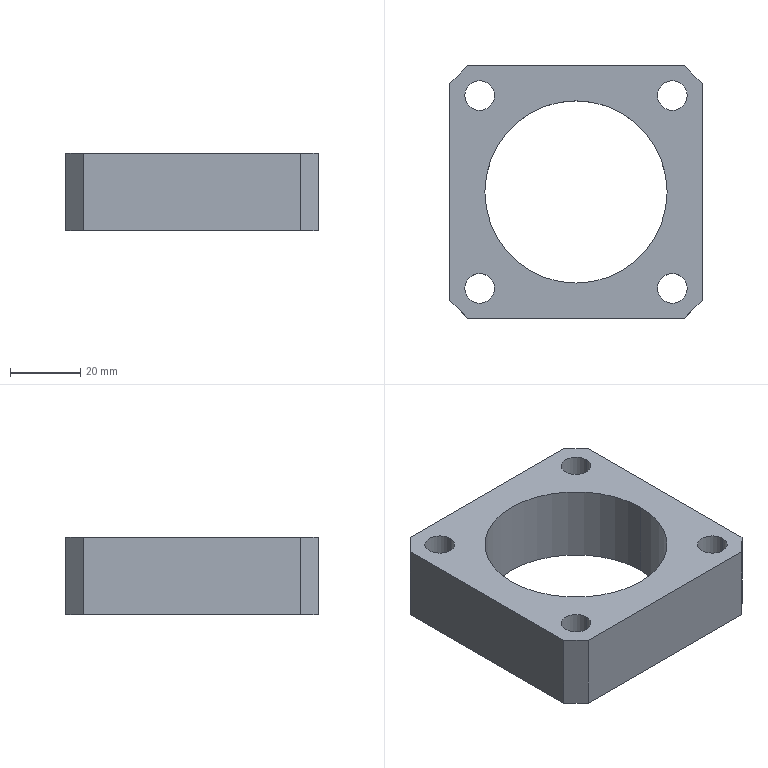Part | 1 solid | 32 faces | box 72 x 72 x 22 mm | volume 58801 mm3 | cylinder 18 | plane 14 | commonest cylinder face diameters 8.5 x8 13 x8 52 x2
STEP:
#1=CARTESIAN_POINT('',(34.,-27.5,-3.));
#2=VERTEX_POINT('',#1);
#3=CARTESIAN_POINT('',(21.,-27.5,-3.));
#4=VERTEX_POINT('',#3);
#5=CARTESIAN_POINT('',(27.5,-27.5,-3.));
#6=DIRECTION('',(0.,0.,-1.));
#7=DIRECTION('',(-1.,0.,0.));
#8=AXIS2_PLACEMENT_3D('',#5,#6,#7);
#9=CIRCLE('',#8,6.5);
#10=EDGE_CURVE('',#2,#4,#9,.T.);
#11=ORIENTED_EDGE('',*,*,#10,.F.);
#12=CARTESIAN_POINT('',(34.,-27.5,-11.));
#13=VERTEX_POINT('',#12);
#14=CARTESIAN_POINT('',(34.,-27.5,-11.));
#15=DIRECTION('',(0.,0.,-1.));
#16=VECTOR('',#15,1000.);
#17=LINE('',#14,#16);
#18=EDGE_CURVE('',#2,#13,#17,.T.);
#19=ORIENTED_EDGE('',*,*,#18,.T.);
#20=CARTESIAN_POINT('',(21.,-27.5,-11.));
#21=VERTEX_POINT('',#20);
#22=CARTESIAN_POINT('',(27.5,-27.5,-11.));
#23=DIRECTION('',(0.,0.,-1.));
#24=DIRECTION('',(-1.,0.,0.));
#25=AXIS2_PLACEMENT_3D('',#22,#23,#24);
#26=CIRCLE('',#25,6.5);
#27=EDGE_CURVE('',#13,#21,#26,.T.);
#28=ORIENTED_EDGE('',*,*,#27,.T.);
#29=CARTESIAN_POINT('',(21.,-27.5,-11.));
#30=DIRECTION('',(0.,0.,-1.));
#31=VECTOR('',#30,1000.);
#32=LINE('',#29,#31);
#33=EDGE_CURVE('',#4,#21,#32,.T.);
#34=ORIENTED_EDGE('',*,*,#33,.F.);
#35=EDGE_LOOP('',(#11,#19,#28,#34));
#36=FACE_OUTER_BOUND('',#35,.T.);
#37=CARTESIAN_POINT('',(27.5,-27.5,-11.));
#38=DIRECTION('',(0.,0.,-1.));
#39=DIRECTION('',(-1.,0.,0.));
#40=AXIS2_PLACEMENT_3D('',#37,#38,#39);
#41=CYLINDRICAL_SURFACE('',#40,6.5);
#42=ADVANCED_FACE('',(#36),#41,.F.);
#43=CARTESIAN_POINT('',(31.75,-27.5,11.));
#44=VERTEX_POINT('',#43);
#45=CARTESIAN_POINT('',(23.25,-27.5,11.));
#46=VERTEX_POINT('',#45);
#47=CARTESIAN_POINT('',(27.5,-27.5,11.));
#48=DIRECTION('',(0.,0.,-1.));
#49=DIRECTION('',(-1.,0.,0.));
#50=AXIS2_PLACEMENT_3D('',#47,#48,#49);
#51=CIRCLE('',#50,4.25);
#52=EDGE_CURVE('',#44,#46,#51,.T.);
#53=ORIENTED_EDGE('',*,*,#52,.F.);
#54=CARTESIAN_POINT('',(31.75,-27.5,-3.));
#55=VERTEX_POINT('',#54);
#56=CARTESIAN_POINT('',(31.75,-27.5,-11.));
#57=DIRECTION('',(0.,0.,-1.));
#58=VECTOR('',#57,1000.);
#59=LINE('',#56,#58);
#60=EDGE_CURVE('',#44,#55,#59,.T.);
#61=ORIENTED_EDGE('',*,*,#60,.T.);
#62=CARTESIAN_POINT('',(23.25,-27.5,-3.));
#63=VERTEX_POINT('',#62);
#64=CARTESIAN_POINT('',(27.5,-27.5,-3.));
#65=DIRECTION('',(0.,0.,-1.));
#66=DIRECTION('',(-1.,0.,0.));
#67=AXIS2_PLACEMENT_3D('',#64,#65,#66);
#68=CIRCLE('',#67,4.25);
#69=EDGE_CURVE('',#55,#63,#68,.T.);
#70=ORIENTED_EDGE('',*,*,#69,.T.);
#71=CARTESIAN_POINT('',(23.25,-27.5,-11.));
#72=DIRECTION('',(0.,0.,-1.));
#73=VECTOR('',#72,1000.);
#74=LINE('',#71,#73);
#75=EDGE_CURVE('',#46,#63,#74,.T.);
#76=ORIENTED_EDGE('',*,*,#75,.F.);
#77=EDGE_LOOP('',(#53,#61,#70,#76));
#78=FACE_OUTER_BOUND('',#77,.T.);
#79=CARTESIAN_POINT('',(27.5,-27.5,-11.));
#80=DIRECTION('',(0.,0.,-1.));
#81=DIRECTION('',(-1.,0.,0.));
#82=AXIS2_PLACEMENT_3D('',#79,#80,#81);
#83=CYLINDRICAL_SURFACE('',#82,4.25);
#84=ADVANCED_FACE('',(#78),#83,.F.);
#85=CARTESIAN_POINT('',(-21.,-27.5,-3.));
#86=VERTEX_POINT('',#85);
#87=CARTESIAN_POINT('',(-34.,-27.5,-3.));
#88=VERTEX_POINT('',#87);
#89=CARTESIAN_POINT('',(-27.5,-27.5,-3.));
#90=DIRECTION('',(0.,0.,-1.));
#91=DIRECTION('',(-1.,0.,0.));
#92=AXIS2_PLACEMENT_3D('',#89,#90,#91);
#93=CIRCLE('',#92,6.5);
#94=EDGE_CURVE('',#86,#88,#93,.T.);
#95=ORIENTED_EDGE('',*,*,#94,.F.);
#96=CARTESIAN_POINT('',(-21.,-27.5,-11.));
#97=VERTEX_POINT('',#96);
#98=CARTESIAN_POINT('',(-21.,-27.5,-11.));
#99=DIRECTION('',(0.,0.,-1.));
#100=VECTOR('',#99,1000.);
#101=LINE('',#98,#100);
#102=EDGE_CURVE('',#86,#97,#101,.T.);
#103=ORIENTED_EDGE('',*,*,#102,.T.);
#104=CARTESIAN_POINT('',(-34.,-27.5,-11.));
#105=VERTEX_POINT('',#104);
#106=CARTESIAN_POINT('',(-27.5,-27.5,-11.));
#107=DIRECTION('',(0.,0.,-1.));
#108=DIRECTION('',(-1.,0.,0.));
#109=AXIS2_PLACEMENT_3D('',#106,#107,#108);
#110=CIRCLE('',#109,6.5);
#111=EDGE_CURVE('',#97,#105,#110,.T.);
#112=ORIENTED_EDGE('',*,*,#111,.T.);
#113=CARTESIAN_POINT('',(-34.,-27.5,-11.));
#114=DIRECTION('',(0.,0.,-1.));
#115=VECTOR('',#114,1000.);
#116=LINE('',#113,#115);
#117=EDGE_CURVE('',#88,#105,#116,.T.);
#118=ORIENTED_EDGE('',*,*,#117,.F.);
#119=EDGE_LOOP('',(#95,#103,#112,#118));
#120=FACE_OUTER_BOUND('',#119,.T.);
#121=CARTESIAN_POINT('',(-27.5,-27.5,-11.));
#122=DIRECTION('',(0.,0.,-1.));
#123=DIRECTION('',(-1.,0.,0.));
#124=AXIS2_PLACEMENT_3D('',#121,#122,#123);
#125=CYLINDRICAL_SURFACE('',#124,6.5);
#126=ADVANCED_FACE('',(#120),#125,.F.);
#127=CARTESIAN_POINT('',(-23.25,-27.5,11.));
#128=VERTEX_POINT('',#127);
#129=CARTESIAN_POINT('',(-31.75,-27.5,11.));
#130=VERTEX_POINT('',#129);
#131=CARTESIAN_POINT('',(-27.5,-27.5,11.));
#132=DIRECTION('',(0.,0.,-1.));
#133=DIRECTION('',(-1.,0.,0.));
#134=AXIS2_PLACEMENT_3D('',#131,#132,#133);
#135=CIRCLE('',#134,4.25);
#136=EDGE_CURVE('',#128,#130,#135,.T.);
#137=ORIENTED_EDGE('',*,*,#136,.F.);
#138=CARTESIAN_POINT('',(-23.25,-27.5,-3.));
#139=VERTEX_POINT('',#138);
#140=CARTESIAN_POINT('',(-23.25,-27.5,-11.));
#141=DIRECTION('',(0.,0.,-1.));
#142=VECTOR('',#141,1000.);
#143=LINE('',#140,#142);
#144=EDGE_CURVE('',#128,#139,#143,.T.);
#145=ORIENTED_EDGE('',*,*,#144,.T.);
#146=CARTESIAN_POINT('',(-31.75,-27.5,-3.));
#147=VERTEX_POINT('',#146);
#148=CARTESIAN_POINT('',(-27.5,-27.5,-3.));
#149=DIRECTION('',(0.,0.,-1.));
#150=DIRECTION('',(-1.,0.,0.));
#151=AXIS2_PLACEMENT_3D('',#148,#149,#150);
#152=CIRCLE('',#151,4.25);
#153=EDGE_CURVE('',#139,#147,#152,.T.);
#154=ORIENTED_EDGE('',*,*,#153,.T.);
#155=CARTESIAN_POINT('',(-31.75,-27.5,-11.));
#156=DIRECTION('',(0.,0.,-1.));
#157=VECTOR('',#156,1000.);
#158=LINE('',#155,#157);
#159=EDGE_CURVE('',#130,#147,#158,.T.);
#160=ORIENTED_EDGE('',*,*,#159,.F.);
#161=EDGE_LOOP('',(#137,#145,#154,#160));
#162=FACE_OUTER_BOUND('',#161,.T.);
#163=CARTESIAN_POINT('',(-27.5,-27.5,-11.));
#164=DIRECTION('',(0.,0.,-1.));
#165=DIRECTION('',(-1.,0.,0.));
#166=AXIS2_PLACEMENT_3D('',#163,#164,#165);
#167=CYLINDRICAL_SURFACE('',#166,4.25);
#168=ADVANCED_FACE('',(#162),#167,.F.);
#169=CARTESIAN_POINT('',(-21.,27.5,-3.));
#170=VERTEX_POINT('',#169);
#171=CARTESIAN_POINT('',(-34.,27.5,-3.));
#172=VERTEX_POINT('',#171);
#173=CARTESIAN_POINT('',(-27.5,27.5,-3.));
#174=DIRECTION('',(0.,0.,-1.));
#175=DIRECTION('',(-1.,0.,0.));
#176=AXIS2_PLACEMENT_3D('',#173,#174,#175);
#177=CIRCLE('',#176,6.5);
#178=EDGE_CURVE('',#170,#172,#177,.T.);
#179=ORIENTED_EDGE('',*,*,#178,.F.);
#180=CARTESIAN_POINT('',(-21.,27.5,-11.));
#181=VERTEX_POINT('',#180);
#182=CARTESIAN_POINT('',(-21.,27.5,-11.));
#183=DIRECTION('',(0.,0.,-1.));
#184=VECTOR('',#183,1000.);
#185=LINE('',#182,#184);
#186=EDGE_CURVE('',#170,#181,#185,.T.);
#187=ORIENTED_EDGE('',*,*,#186,.T.);
#188=CARTESIAN_POINT('',(-34.,27.5,-11.));
#189=VERTEX_POINT('',#188);
#190=CARTESIAN_POINT('',(-27.5,27.5,-11.));
#191=DIRECTION('',(0.,0.,-1.));
#192=DIRECTION('',(-1.,0.,0.));
#193=AXIS2_PLACEMENT_3D('',#190,#191,#192);
#194=CIRCLE('',#193,6.5);
#195=EDGE_CURVE('',#181,#189,#194,.T.);
#196=ORIENTED_EDGE('',*,*,#195,.T.);
#197=CARTESIAN_POINT('',(-34.,27.5,-11.));
#198=DIRECTION('',(0.,0.,-1.));
#199=VECTOR('',#198,1000.);
#200=LINE('',#197,#199);
#201=EDGE_CURVE('',#172,#189,#200,.T.);
#202=ORIENTED_EDGE('',*,*,#201,.F.);
#203=EDGE_LOOP('',(#179,#187,#196,#202));
#204=FACE_OUTER_BOUND('',#203,.T.);
#205=CARTESIAN_POINT('',(-27.5,27.5,-11.));
#206=DIRECTION('',(0.,0.,-1.));
#207=DIRECTION('',(-1.,0.,0.));
#208=AXIS2_PLACEMENT_3D('',#205,#206,#207);
#209=CYLINDRICAL_SURFACE('',#208,6.5);
#210=ADVANCED_FACE('',(#204),#209,.F.);
#211=CARTESIAN_POINT('',(-23.25,27.5,11.));
#212=VERTEX_POINT('',#211);
#213=CARTESIAN_POINT('',(-31.75,27.5,11.));
#214=VERTEX_POINT('',#213);
#215=CARTESIAN_POINT('',(-27.5,27.5,11.));
#216=DIRECTION('',(0.,0.,-1.));
#217=DIRECTION('',(-1.,0.,0.));
#218=AXIS2_PLACEMENT_3D('',#215,#216,#217);
#219=CIRCLE('',#218,4.25);
#220=EDGE_CURVE('',#212,#214,#219,.T.);
#221=ORIENTED_EDGE('',*,*,#220,.F.);
#222=CARTESIAN_POINT('',(-23.25,27.5,-3.));
#223=VERTEX_POINT('',#222);
#224=CARTESIAN_POINT('',(-23.25,27.5,-11.));
#225=DIRECTION('',(0.,0.,-1.));
#226=VECTOR('',#225,1000.);
#227=LINE('',#224,#226);
#228=EDGE_CURVE('',#212,#223,#227,.T.);
#229=ORIENTED_EDGE('',*,*,#228,.T.);
#230=CARTESIAN_POINT('',(-31.75,27.5,-3.));
#231=VERTEX_POINT('',#230);
#232=CARTESIAN_POINT('',(-27.5,27.5,-3.));
#233=DIRECTION('',(0.,0.,-1.));
#234=DIRECTION('',(-1.,0.,0.));
#235=AXIS2_PLACEMENT_3D('',#232,#233,#234);
#236=CIRCLE('',#235,4.25);
#237=EDGE_CURVE('',#223,#231,#236,.T.);
#238=ORIENTED_EDGE('',*,*,#237,.T.);
#239=CARTESIAN_POINT('',(-31.75,27.5,-11.));
#240=DIRECTION('',(0.,0.,-1.));
#241=VECTOR('',#240,1000.);
#242=LINE('',#239,#241);
#243=EDGE_CURVE('',#214,#231,#242,.T.);
#244=ORIENTED_EDGE('',*,*,#243,.F.);
#245=EDGE_LOOP('',(#221,#229,#238,#244));
#246=FACE_OUTER_BOUND('',#245,.T.);
#247=CARTESIAN_POINT('',(-27.5,27.5,-11.));
#248=DIRECTION('',(0.,0.,-1.));
#249=DIRECTION('',(-1.,0.,0.));
#250=AXIS2_PLACEMENT_3D('',#247,#248,#249);
#251=CYLINDRICAL_SURFACE('',#250,4.25);
#252=ADVANCED_FACE('',(#246),#251,.F.);
#253=CARTESIAN_POINT('',(34.,27.5,-3.));
#254=VERTEX_POINT('',#253);
#255=CARTESIAN_POINT('',(21.,27.5,-3.));
#256=VERTEX_POINT('',#255);
#257=CARTESIAN_POINT('',(27.5,27.5,-3.));
#258=DIRECTION('',(0.,0.,-1.));
#259=DIRECTION('',(-1.,0.,0.));
#260=AXIS2_PLACEMENT_3D('',#257,#258,#259);
#261=CIRCLE('',#260,6.5);
#262=EDGE_CURVE('',#254,#256,#261,.T.);
#263=ORIENTED_EDGE('',*,*,#262,.F.);
#264=CARTESIAN_POINT('',(34.,27.5,-11.));
#265=VERTEX_POINT('',#264);
#266=CARTESIAN_POINT('',(34.,27.5,-11.));
#267=DIRECTION('',(0.,0.,-1.));
#268=VECTOR('',#267,1000.);
#269=LINE('',#266,#268);
#270=EDGE_CURVE('',#254,#265,#269,.T.);
#271=ORIENTED_EDGE('',*,*,#270,.T.);
#272=CARTESIAN_POINT('',(21.,27.5,-11.));
#273=VERTEX_POINT('',#272);
#274=CARTESIAN_POINT('',(27.5,27.5,-11.));
#275=DIRECTION('',(0.,0.,-1.));
#276=DIRECTION('',(-1.,0.,0.));
#277=AXIS2_PLACEMENT_3D('',#274,#275,#276);
#278=CIRCLE('',#277,6.5);
#279=EDGE_CURVE('',#265,#273,#278,.T.);
#280=ORIENTED_EDGE('',*,*,#279,.T.);
#281=CARTESIAN_POINT('',(21.,27.5,-11.));
#282=DIRECTION('',(0.,0.,-1.));
#283=VECTOR('',#282,1000.);
#284=LINE('',#281,#283);
#285=EDGE_CURVE('',#256,#273,#284,.T.);
#286=ORIENTED_EDGE('',*,*,#285,.F.);
#287=EDGE_LOOP('',(#263,#271,#280,#286));
#288=FACE_OUTER_BOUND('',#287,.T.);
#289=CARTESIAN_POINT('',(27.5,27.5,-11.));
#290=DIRECTION('',(0.,0.,-1.));
#291=DIRECTION('',(-1.,0.,0.));
#292=AXIS2_PLACEMENT_3D('',#289,#290,#291);
#293=CYLINDRICAL_SURFACE('',#292,6.5);
#294=ADVANCED_FACE('',(#288),#293,.F.);
#295=CARTESIAN_POINT('',(31.75,27.5,11.));
#296=VERTEX_POINT('',#295);
#297=CARTESIAN_POINT('',(23.25,27.5,11.));
#298=VERTEX_POINT('',#297);
#299=CARTESIAN_POINT('',(27.5,27.5,11.));
#300=DIRECTION('',(0.,0.,-1.));
#301=DIRECTION('',(-1.,0.,0.));
#302=AXIS2_PLACEMENT_3D('',#299,#300,#301);
#303=CIRCLE('',#302,4.25);
#304=EDGE_CURVE('',#296,#298,#303,.T.);
#305=ORIENTED_EDGE('',*,*,#304,.F.);
#306=CARTESIAN_POINT('',(31.75,27.5,-3.));
#307=VERTEX_POINT('',#306);
#308=CARTESIAN_POINT('',(31.75,27.5,-11.));
#309=DIRECTION('',(0.,0.,-1.));
#310=VECTOR('',#309,1000.);
#311=LINE('',#308,#310);
#312=EDGE_CURVE('',#296,#307,#311,.T.);
#313=ORIENTED_EDGE('',*,*,#312,.T.);
#314=CARTESIAN_POINT('',(23.25,27.5,-3.));
#315=VERTEX_POINT('',#314);
#316=CARTESIAN_POINT('',(27.5,27.5,-3.));
#317=DIRECTION('',(0.,0.,-1.));
#318=DIRECTION('',(-1.,0.,0.));
#319=AXIS2_PLACEMENT_3D('',#316,#317,#318);
#320=CIRCLE('',#319,4.25);
#321=EDGE_CURVE('',#307,#315,#320,.T.);
#322=ORIENTED_EDGE('',*,*,#321,.T.);
#323=CARTESIAN_POINT('',(23.25,27.5,-11.));
#324=DIRECTION('',(0.,0.,-1.));
#325=VECTOR('',#324,1000.);
#326=LINE('',#323,#325);
#327=EDGE_CURVE('',#298,#315,#326,.T.);
#328=ORIENTED_EDGE('',*,*,#327,.F.);
#329=EDGE_LOOP('',(#305,#313,#322,#328));
#330=FACE_OUTER_BOUND('',#329,.T.);
#331=CARTESIAN_POINT('',(27.5,27.5,-11.));
#332=DIRECTION('',(0.,0.,-1.));
#333=DIRECTION('',(-1.,0.,0.));
#334=AXIS2_PLACEMENT_3D('',#331,#332,#333);
#335=CYLINDRICAL_SURFACE('',#334,4.25);
#336=ADVANCED_FACE('',(#330),#335,.F.);
#337=CARTESIAN_POINT('',(26.,0.,11.));
#338=VERTEX_POINT('',#337);
#339=CARTESIAN_POINT('',(-26.,0.,11.));
#340=VERTEX_POINT('',#339);
#341=CARTESIAN_POINT('',(0.,0.,11.));
#342=DIRECTION('',(0.,0.,-1.));
#343=DIRECTION('',(-1.,0.,0.));
#344=AXIS2_PLACEMENT_3D('',#341,#342,#343);
#345=CIRCLE('',#344,26.);
#346=EDGE_CURVE('',#338,#340,#345,.T.);
#347=ORIENTED_EDGE('',*,*,#346,.F.);
#348=CARTESIAN_POINT('',(26.,0.,-11.));
#349=VERTEX_POINT('',#348);
#350=CARTESIAN_POINT('',(26.,0.,-11.));
#351=DIRECTION('',(0.,0.,-1.));
#352=VECTOR('',#351,1000.);
#353=LINE('',#350,#352);
#354=EDGE_CURVE('',#338,#349,#353,.T.);
#355=ORIENTED_EDGE('',*,*,#354,.T.);
#356=CARTESIAN_POINT('',(-26.,0.,-11.));
#357=VERTEX_POINT('',#356);
#358=CARTESIAN_POINT('',(0.,0.,-11.));
#359=DIRECTION('',(0.,0.,-1.));
#360=DIRECTION('',(-1.,0.,0.));
#361=AXIS2_PLACEMENT_3D('',#358,#359,#360);
#362=CIRCLE('',#361,26.);
#363=EDGE_CURVE('',#349,#357,#362,.T.);
#364=ORIENTED_EDGE('',*,*,#363,.T.);
#365=CARTESIAN_POINT('',(-26.,0.,-11.));
#366=DIRECTION('',(0.,0.,-1.));
#367=VECTOR('',#366,1000.);
#368=LINE('',#365,#367);
#369=EDGE_CURVE('',#340,#357,#368,.T.);
#370=ORIENTED_EDGE('',*,*,#369,.F.);
#371=EDGE_LOOP('',(#347,#355,#364,#370));
#372=FACE_OUTER_BOUND('',#371,.T.);
#373=CARTESIAN_POINT('',(0.,0.,-11.));
#374=DIRECTION('',(0.,0.,-1.));
#375=DIRECTION('',(-1.,0.,0.));
#376=AXIS2_PLACEMENT_3D('',#373,#374,#375);
#377=CYLINDRICAL_SURFACE('',#376,26.);
#378=ADVANCED_FACE('',(#372),#377,.F.);
#379=CARTESIAN_POINT('',(-31.,36.,-11.));
#380=VERTEX_POINT('',#379);
#381=CARTESIAN_POINT('',(31.,36.,-11.));
#382=VERTEX_POINT('',#381);
#383=CARTESIAN_POINT('',(-36.,36.,-11.));
#384=DIRECTION('',(1.,0.,0.));
#385=VECTOR('',#384,1000.);
#386=LINE('',#383,#385);
#387=EDGE_CURVE('',#380,#382,#386,.T.);
#388=ORIENTED_EDGE('',*,*,#387,.F.);
#389=CARTESIAN_POINT('',(-31.,36.,11.));
#390=VERTEX_POINT('',#389);
#391=CARTESIAN_POINT('',(-31.,36.,11.));
#392=DIRECTION('',(0.,0.,1.));
#393=VECTOR('',#392,1000.);
#394=LINE('',#391,#393);
#395=EDGE_CURVE('',#380,#390,#394,.T.);
#396=ORIENTED_EDGE('',*,*,#395,.T.);
#397=CARTESIAN_POINT('',(31.,36.,11.));
#398=VERTEX_POINT('',#397);
#399=CARTESIAN_POINT('',(-36.,36.,11.));
#400=DIRECTION('',(1.,0.,0.));
#401=VECTOR('',#400,1000.);
#402=LINE('',#399,#401);
#403=EDGE_CURVE('',#390,#398,#402,.T.);
#404=ORIENTED_EDGE('',*,*,#403,.T.);
#405=CARTESIAN_POINT('',(31.,36.,11.));
#406=DIRECTION('',(0.,0.,-1.));
#407=VECTOR('',#406,1000.);
#408=LINE('',#405,#407);
#409=EDGE_CURVE('',#398,#382,#408,.T.);
#410=ORIENTED_EDGE('',*,*,#409,.T.);
#411=EDGE_LOOP('',(#388,#396,#404,#410));
#412=FACE_OUTER_BOUND('',#411,.T.);
#413=CARTESIAN_POINT('',(-36.,36.,11.));
#414=DIRECTION('',(0.,1.,0.));
#415=DIRECTION('',(0.,0.,1.));
#416=AXIS2_PLACEMENT_3D('',#413,#414,#415);
#417=PLANE('',#416);
#418=ADVANCED_FACE('',(#412),#417,.T.);
#419=CARTESIAN_POINT('',(-36.,-31.,-11.));
#420=VERTEX_POINT('',#419);
#421=CARTESIAN_POINT('',(-36.,31.,-11.));
#422=VERTEX_POINT('',#421);
#423=CARTESIAN_POINT('',(-36.,-36.,-11.));
#424=DIRECTION('',(0.,1.,0.));
#425=VECTOR('',#424,1000.);
#426=LINE('',#423,#425);
#427=EDGE_CURVE('',#420,#422,#426,.T.);
#428=ORIENTED_EDGE('',*,*,#427,.F.);
#429=CARTESIAN_POINT('',(-36.,-31.,11.));
#430=VERTEX_POINT('',#429);
#431=CARTESIAN_POINT('',(-36.,-31.,11.));
#432=DIRECTION('',(0.,0.,1.));
#433=VECTOR('',#432,1000.);
#434=LINE('',#431,#433);
#435=EDGE_CURVE('',#420,#430,#434,.T.);
#436=ORIENTED_EDGE('',*,*,#435,.T.);
#437=CARTESIAN_POINT('',(-36.,31.,11.));
#438=VERTEX_POINT('',#437);
#439=CARTESIAN_POINT('',(-36.,-36.,11.));
#440=DIRECTION('',(0.,1.,0.));
#441=VECTOR('',#440,1000.);
#442=LINE('',#439,#441);
#443=EDGE_CURVE('',#430,#438,#442,.T.);
#444=ORIENTED_EDGE('',*,*,#443,.T.);
#445=CARTESIAN_POINT('',(-36.,31.,11.));
#446=DIRECTION('',(0.,0.,-1.));
#447=VECTOR('',#446,1000.);
#448=LINE('',#445,#447);
#449=EDGE_CURVE('',#438,#422,#448,.T.);
#450=ORIENTED_EDGE('',*,*,#449,.T.);
#451=EDGE_LOOP('',(#428,#436,#444,#450));
#452=FACE_OUTER_BOUND('',#451,.T.);
#453=CARTESIAN_POINT('',(-36.,-36.,11.));
#454=DIRECTION('',(-1.,0.,0.));
#455=DIRECTION('',(0.,-1.,0.));
#456=AXIS2_PLACEMENT_3D('',#453,#454,#455);
#457=PLANE('',#456);
#458=ADVANCED_FACE('',(#452),#457,.T.);
#459=CARTESIAN_POINT('',(31.,-36.,11.));
#460=VERTEX_POINT('',#459);
#461=CARTESIAN_POINT('',(-31.,-36.,11.));
#462=VERTEX_POINT('',#461);
#463=CARTESIAN_POINT('',(36.,-36.,11.));
#464=DIRECTION('',(-1.,0.,0.));
#465=VECTOR('',#464,1000.);
#466=LINE('',#463,#465);
#467=EDGE_CURVE('',#460,#462,#466,.T.);
#468=ORIENTED_EDGE('',*,*,#467,.T.);
#469=CARTESIAN_POINT('',(-31.,-36.,-11.));
#470=VERTEX_POINT('',#469);
#471=CARTESIAN_POINT('',(-31.,-36.,11.));
#472=DIRECTION('',(0.,0.,-1.));
#473=VECTOR('',#472,1000.);
#474=LINE('',#471,#473);
#475=EDGE_CURVE('',#462,#470,#474,.T.);
#476=ORIENTED_EDGE('',*,*,#475,.T.);
#477=CARTESIAN_POINT('',(31.,-36.,-11.));
#478=VERTEX_POINT('',#477);
#479=CARTESIAN_POINT('',(36.,-36.,-11.));
#480=DIRECTION('',(-1.,0.,0.));
#481=VECTOR('',#480,1000.);
#482=LINE('',#479,#481);
#483=EDGE_CURVE('',#478,#470,#482,.T.);
#484=ORIENTED_EDGE('',*,*,#483,.F.);
#485=CARTESIAN_POINT('',(31.,-36.,11.));
#486=DIRECTION('',(0.,0.,1.));
#487=VECTOR('',#486,1000.);
#488=LINE('',#485,#487);
#489=EDGE_CURVE('',#478,#460,#488,.T.);
#490=ORIENTED_EDGE('',*,*,#489,.T.);
#491=EDGE_LOOP('',(#468,#476,#484,#490));
#492=FACE_OUTER_BOUND('',#491,.T.);
#493=CARTESIAN_POINT('',(36.,-36.,11.));
#494=DIRECTION('',(0.,-1.,0.));
#495=DIRECTION('',(0.,0.,-1.));
#496=AXIS2_PLACEMENT_3D('',#493,#494,#495);
#497=PLANE('',#496);
#498=ADVANCED_FACE('',(#492),#497,.T.);
#499=CARTESIAN_POINT('',(36.,31.,11.));
#500=VERTEX_POINT('',#499);
#501=CARTESIAN_POINT('',(36.,-31.,11.));
#502=VERTEX_POINT('',#501);
#503=CARTESIAN_POINT('',(36.,36.,11.));
#504=DIRECTION('',(0.,-1.,0.));
#505=VECTOR('',#504,1000.);
#506=LINE('',#503,#505);
#507=EDGE_CURVE('',#500,#502,#506,.T.);
#508=ORIENTED_EDGE('',*,*,#507,.T.);
#509=CARTESIAN_POINT('',(36.,-31.,-11.));
#510=VERTEX_POINT('',#509);
#511=CARTESIAN_POINT('',(36.,-31.,11.));
#512=DIRECTION('',(0.,0.,-1.));
#513=VECTOR('',#512,1000.);
#514=LINE('',#511,#513);
#515=EDGE_CURVE('',#502,#510,#514,.T.);
#516=ORIENTED_EDGE('',*,*,#515,.T.);
#517=CARTESIAN_POINT('',(36.,31.,-11.));
#518=VERTEX_POINT('',#517);
#519=CARTESIAN_POINT('',(36.,36.,-11.));
#520=DIRECTION('',(0.,-1.,0.));
#521=VECTOR('',#520,1000.);
#522=LINE('',#519,#521);
#523=EDGE_CURVE('',#518,#510,#522,.T.);
#524=ORIENTED_EDGE('',*,*,#523,.F.);
#525=CARTESIAN_POINT('',(36.,31.,11.));
#526=DIRECTION('',(0.,0.,1.));
#527=VECTOR('',#526,1000.);
#528=LINE('',#525,#527);
#529=EDGE_CURVE('',#518,#500,#528,.T.);
#530=ORIENTED_EDGE('',*,*,#529,.T.);
#531=EDGE_LOOP('',(#508,#516,#524,#530));
#532=FACE_OUTER_BOUND('',#531,.T.);
#533=CARTESIAN_POINT('',(36.,36.,11.));
#534=DIRECTION('',(1.,0.,0.));
#535=DIRECTION('',(0.,1.,0.));
#536=AXIS2_PLACEMENT_3D('',#533,#534,#535);
#537=PLANE('',#536);
#538=ADVANCED_FACE('',(#532),#537,.T.);
#539=CARTESIAN_POINT('',(27.5,-27.5,11.));
#540=DIRECTION('',(0.,0.,-1.));
#541=DIRECTION('',(-1.,0.,0.));
#542=AXIS2_PLACEMENT_3D('',#539,#540,#541);
#543=CIRCLE('',#542,4.25);
#544=EDGE_CURVE('',#46,#44,#543,.T.);
#545=ORIENTED_EDGE('',*,*,#544,.T.);
#546=ORIENTED_EDGE('',*,*,#52,.T.);
#547=EDGE_LOOP('',(#545,#546));
#548=FACE_BOUND('',#547,.T.);
#549=CARTESIAN_POINT('',(-27.5,-27.5,11.));
#550=DIRECTION('',(0.,0.,-1.));
#551=DIRECTION('',(-1.,0.,0.));
#552=AXIS2_PLACEMENT_3D('',#549,#550,#551);
#553=CIRCLE('',#552,4.25);
#554=EDGE_CURVE('',#130,#128,#553,.T.);
#555=ORIENTED_EDGE('',*,*,#554,.T.);
#556=ORIENTED_EDGE('',*,*,#136,.T.);
#557=EDGE_LOOP('',(#555,#556));
#558=FACE_BOUND('',#557,.T.);
#559=CARTESIAN_POINT('',(-27.5,27.5,11.));
#560=DIRECTION('',(0.,0.,-1.));
#561=DIRECTION('',(-1.,0.,0.));
#562=AXIS2_PLACEMENT_3D('',#559,#560,#561);
#563=CIRCLE('',#562,4.25);
#564=EDGE_CURVE('',#214,#212,#563,.T.);
#565=ORIENTED_EDGE('',*,*,#564,.T.);
#566=ORIENTED_EDGE('',*,*,#220,.T.);
#567=EDGE_LOOP('',(#565,#566));
#568=FACE_BOUND('',#567,.T.);
#569=CARTESIAN_POINT('',(27.5,27.5,11.));
#570=DIRECTION('',(0.,0.,-1.));
#571=DIRECTION('',(-1.,0.,0.));
#572=AXIS2_PLACEMENT_3D('',#569,#570,#571);
#573=CIRCLE('',#572,4.25);
#574=EDGE_CURVE('',#298,#296,#573,.T.);
#575=ORIENTED_EDGE('',*,*,#574,.T.);
#576=ORIENTED_EDGE('',*,*,#304,.T.);
#577=EDGE_LOOP('',(#575,#576));
#578=FACE_BOUND('',#577,.T.);
#579=CARTESIAN_POINT('',(0.,0.,11.));
#580=DIRECTION('',(0.,0.,-1.));
#581=DIRECTION('',(-1.,0.,0.));
#582=AXIS2_PLACEMENT_3D('',#579,#580,#581);
#583=CIRCLE('',#582,26.);
#584=EDGE_CURVE('',#340,#338,#583,.T.);
#585=ORIENTED_EDGE('',*,*,#584,.T.);
#586=ORIENTED_EDGE('',*,*,#346,.T.);
#587=EDGE_LOOP('',(#585,#586));
#588=FACE_BOUND('',#587,.T.);
#589=ORIENTED_EDGE('',*,*,#443,.F.);
#590=CARTESIAN_POINT('',(-31.,-36.,11.));
#591=DIRECTION('',(0.7071,-0.7071,0.));
#592=VECTOR('',#591,1000.);
#593=LINE('',#590,#592);
#594=EDGE_CURVE('',#430,#462,#593,.T.);
#595=ORIENTED_EDGE('',*,*,#594,.T.);
#596=ORIENTED_EDGE('',*,*,#467,.F.);
#597=CARTESIAN_POINT('',(36.,-31.,11.));
#598=DIRECTION('',(0.7071,0.7071,0.));
#599=VECTOR('',#598,1000.);
#600=LINE('',#597,#599);
#601=EDGE_CURVE('',#460,#502,#600,.T.);
#602=ORIENTED_EDGE('',*,*,#601,.T.);
#603=ORIENTED_EDGE('',*,*,#507,.F.);
#604=CARTESIAN_POINT('',(31.,36.,11.));
#605=DIRECTION('',(-0.7071,0.7071,0.));
#606=VECTOR('',#605,1000.);
#607=LINE('',#604,#606);
#608=EDGE_CURVE('',#500,#398,#607,.T.);
#609=ORIENTED_EDGE('',*,*,#608,.T.);
#610=ORIENTED_EDGE('',*,*,#403,.F.);
#611=CARTESIAN_POINT('',(-36.,31.,11.));
#612=DIRECTION('',(-0.7071,-0.7071,0.));
#613=VECTOR('',#612,1000.);
#614=LINE('',#611,#613);
#615=EDGE_CURVE('',#390,#438,#614,.T.);
#616=ORIENTED_EDGE('',*,*,#615,.T.);
#617=EDGE_LOOP('',(#589,#595,#596,#602,#603,#609,#610,#616));
#618=FACE_OUTER_BOUND('',#617,.T.);
#619=CARTESIAN_POINT('',(0.,0.,11.));
#620=DIRECTION('',(0.,0.,-1.));
#621=DIRECTION('',(-1.,0.,0.));
#622=AXIS2_PLACEMENT_3D('',#619,#620,#621);
#623=PLANE('',#622);
#624=ADVANCED_FACE('',(#548,#558,#568,#578,#588,#618),#623,.F.);
#625=CARTESIAN_POINT('',(27.5,-27.5,-11.));
#626=DIRECTION('',(0.,0.,-1.));
#627=DIRECTION('',(-1.,0.,0.));
#628=AXIS2_PLACEMENT_3D('',#625,#626,#627);
#629=CIRCLE('',#628,6.5);
#630=EDGE_CURVE('',#21,#13,#629,.T.);
#631=ORIENTED_EDGE('',*,*,#630,.F.);
#632=ORIENTED_EDGE('',*,*,#27,.F.);
#633=EDGE_LOOP('',(#631,#632));
#634=FACE_BOUND('',#633,.T.);
#635=CARTESIAN_POINT('',(-27.5,-27.5,-11.));
#636=DIRECTION('',(0.,0.,-1.));
#637=DIRECTION('',(-1.,0.,0.));
#638=AXIS2_PLACEMENT_3D('',#635,#636,#637);
#639=CIRCLE('',#638,6.5);
#640=EDGE_CURVE('',#105,#97,#639,.T.);
#641=ORIENTED_EDGE('',*,*,#640,.F.);
#642=ORIENTED_EDGE('',*,*,#111,.F.);
#643=EDGE_LOOP('',(#641,#642));
#644=FACE_BOUND('',#643,.T.);
#645=CARTESIAN_POINT('',(-27.5,27.5,-11.));
#646=DIRECTION('',(0.,0.,-1.));
#647=DIRECTION('',(-1.,0.,0.));
#648=AXIS2_PLACEMENT_3D('',#645,#646,#647);
#649=CIRCLE('',#648,6.5);
#650=EDGE_CURVE('',#189,#181,#649,.T.);
#651=ORIENTED_EDGE('',*,*,#650,.F.);
#652=ORIENTED_EDGE('',*,*,#195,.F.);
#653=EDGE_LOOP('',(#651,#652));
#654=FACE_BOUND('',#653,.T.);
#655=CARTESIAN_POINT('',(27.5,27.5,-11.));
#656=DIRECTION('',(0.,0.,-1.));
#657=DIRECTION('',(-1.,0.,0.));
#658=AXIS2_PLACEMENT_3D('',#655,#656,#657);
#659=CIRCLE('',#658,6.5);
#660=EDGE_CURVE('',#273,#265,#659,.T.);
#661=ORIENTED_EDGE('',*,*,#660,.F.);
#662=ORIENTED_EDGE('',*,*,#279,.F.);
#663=EDGE_LOOP('',(#661,#662));
#664=FACE_BOUND('',#663,.T.);
#665=CARTESIAN_POINT('',(0.,0.,-11.));
#666=DIRECTION('',(0.,0.,-1.));
#667=DIRECTION('',(-1.,0.,0.));
#668=AXIS2_PLACEMENT_3D('',#665,#666,#667);
#669=CIRCLE('',#668,26.);
#670=EDGE_CURVE('',#357,#349,#669,.T.);
#671=ORIENTED_EDGE('',*,*,#670,.F.);
#672=ORIENTED_EDGE('',*,*,#363,.F.);
#673=EDGE_LOOP('',(#671,#672));
#674=FACE_BOUND('',#673,.T.);
#675=ORIENTED_EDGE('',*,*,#483,.T.);
#676=CARTESIAN_POINT('',(-33.5,-33.5,-11.));
#677=DIRECTION('',(-0.7071,0.7071,0.));
#678=VECTOR('',#677,1000.);
#679=LINE('',#676,#678);
#680=EDGE_CURVE('',#470,#420,#679,.T.);
#681=ORIENTED_EDGE('',*,*,#680,.T.);
#682=ORIENTED_EDGE('',*,*,#427,.T.);
#683=CARTESIAN_POINT('',(-33.5,33.5,-11.));
#684=DIRECTION('',(0.7071,0.7071,0.));
#685=VECTOR('',#684,1000.);
#686=LINE('',#683,#685);
#687=EDGE_CURVE('',#422,#380,#686,.T.);
#688=ORIENTED_EDGE('',*,*,#687,.T.);
#689=ORIENTED_EDGE('',*,*,#387,.T.);
#690=CARTESIAN_POINT('',(33.5,33.5,-11.));
#691=DIRECTION('',(0.7071,-0.7071,0.));
#692=VECTOR('',#691,1000.);
#693=LINE('',#690,#692);
#694=EDGE_CURVE('',#382,#518,#693,.T.);
#695=ORIENTED_EDGE('',*,*,#694,.T.);
#696=ORIENTED_EDGE('',*,*,#523,.T.);
#697=CARTESIAN_POINT('',(33.5,-33.5,-11.));
#698=DIRECTION('',(-0.7071,-0.7071,0.));
#699=VECTOR('',#698,1000.);
#700=LINE('',#697,#699);
#701=EDGE_CURVE('',#510,#478,#700,.T.);
#702=ORIENTED_EDGE('',*,*,#701,.T.);
#703=EDGE_LOOP('',(#675,#681,#682,#688,#689,#695,#696,#702));
#704=FACE_OUTER_BOUND('',#703,.T.);
#705=CARTESIAN_POINT('',(0.,0.,-11.));
#706=DIRECTION('',(0.,0.,-1.));
#707=DIRECTION('',(-1.,0.,0.));
#708=AXIS2_PLACEMENT_3D('',#705,#706,#707);
#709=PLANE('',#708);
#710=ADVANCED_FACE('',(#634,#644,#654,#664,#674,#704),#709,.T.);
#711=ORIENTED_EDGE('',*,*,#354,.F.);
#712=ORIENTED_EDGE('',*,*,#584,.F.);
#713=ORIENTED_EDGE('',*,*,#369,.T.);
#714=ORIENTED_EDGE('',*,*,#670,.T.);
#715=EDGE_LOOP('',(#711,#712,#713,#714));
#716=FACE_OUTER_BOUND('',#715,.T.);
#717=CARTESIAN_POINT('',(0.,0.,-11.));
#718=DIRECTION('',(0.,0.,-1.));
#719=DIRECTION('',(-1.,0.,0.));
#720=AXIS2_PLACEMENT_3D('',#717,#718,#719);
#721=CYLINDRICAL_SURFACE('',#720,26.);
#722=ADVANCED_FACE('',(#716),#721,.F.);
#723=ORIENTED_EDGE('',*,*,#312,.F.);
#724=ORIENTED_EDGE('',*,*,#574,.F.);
#725=ORIENTED_EDGE('',*,*,#327,.T.);
#726=CARTESIAN_POINT('',(27.5,27.5,-3.));
#727=DIRECTION('',(0.,0.,-1.));
#728=DIRECTION('',(-1.,0.,0.));
#729=AXIS2_PLACEMENT_3D('',#726,#727,#728);
#730=CIRCLE('',#729,4.25);
#731=EDGE_CURVE('',#315,#307,#730,.T.);
#732=ORIENTED_EDGE('',*,*,#731,.T.);
#733=EDGE_LOOP('',(#723,#724,#725,#732));
#734=FACE_OUTER_BOUND('',#733,.T.);
#735=CARTESIAN_POINT('',(27.5,27.5,-11.));
#736=DIRECTION('',(0.,0.,-1.));
#737=DIRECTION('',(-1.,0.,0.));
#738=AXIS2_PLACEMENT_3D('',#735,#736,#737);
#739=CYLINDRICAL_SURFACE('',#738,4.25);
#740=ADVANCED_FACE('',(#734),#739,.F.);
#741=ORIENTED_EDGE('',*,*,#731,.F.);
#742=ORIENTED_EDGE('',*,*,#321,.F.);
#743=EDGE_LOOP('',(#741,#742));
#744=FACE_BOUND('',#743,.T.);
#745=CARTESIAN_POINT('',(27.5,27.5,-3.));
#746=DIRECTION('',(0.,0.,-1.));
#747=DIRECTION('',(-1.,0.,0.));
#748=AXIS2_PLACEMENT_3D('',#745,#746,#747);
#749=CIRCLE('',#748,6.5);
#750=EDGE_CURVE('',#256,#254,#749,.T.);
#751=ORIENTED_EDGE('',*,*,#750,.T.);
#752=ORIENTED_EDGE('',*,*,#262,.T.);
#753=EDGE_LOOP('',(#751,#752));
#754=FACE_OUTER_BOUND('',#753,.T.);
#755=CARTESIAN_POINT('',(31.75,27.5,-3.));
#756=DIRECTION('',(0.,0.,1.));
#757=DIRECTION('',(1.,0.,0.));
#758=AXIS2_PLACEMENT_3D('',#755,#756,#757);
#759=PLANE('',#758);
#760=ADVANCED_FACE('',(#744,#754),#759,.F.);
#761=ORIENTED_EDGE('',*,*,#270,.F.);
#762=ORIENTED_EDGE('',*,*,#750,.F.);
#763=ORIENTED_EDGE('',*,*,#285,.T.);
#764=ORIENTED_EDGE('',*,*,#660,.T.);
#765=EDGE_LOOP('',(#761,#762,#763,#764));
#766=FACE_OUTER_BOUND('',#765,.T.);
#767=CARTESIAN_POINT('',(27.5,27.5,-11.));
#768=DIRECTION('',(0.,0.,-1.));
#769=DIRECTION('',(-1.,0.,0.));
#770=AXIS2_PLACEMENT_3D('',#767,#768,#769);
#771=CYLINDRICAL_SURFACE('',#770,6.5);
#772=ADVANCED_FACE('',(#766),#771,.F.);
#773=ORIENTED_EDGE('',*,*,#228,.F.);
#774=ORIENTED_EDGE('',*,*,#564,.F.);
#775=ORIENTED_EDGE('',*,*,#243,.T.);
#776=CARTESIAN_POINT('',(-27.5,27.5,-3.));
#777=DIRECTION('',(0.,0.,-1.));
#778=DIRECTION('',(-1.,0.,0.));
#779=AXIS2_PLACEMENT_3D('',#776,#777,#778);
#780=CIRCLE('',#779,4.25);
#781=EDGE_CURVE('',#231,#223,#780,.T.);
#782=ORIENTED_EDGE('',*,*,#781,.T.);
#783=EDGE_LOOP('',(#773,#774,#775,#782));
#784=FACE_OUTER_BOUND('',#783,.T.);
#785=CARTESIAN_POINT('',(-27.5,27.5,-11.));
#786=DIRECTION('',(0.,0.,-1.));
#787=DIRECTION('',(-1.,0.,0.));
#788=AXIS2_PLACEMENT_3D('',#785,#786,#787);
#789=CYLINDRICAL_SURFACE('',#788,4.25);
#790=ADVANCED_FACE('',(#784),#789,.F.);
#791=ORIENTED_EDGE('',*,*,#781,.F.);
#792=ORIENTED_EDGE('',*,*,#237,.F.);
#793=EDGE_LOOP('',(#791,#792));
#794=FACE_BOUND('',#793,.T.);
#795=CARTESIAN_POINT('',(-27.5,27.5,-3.));
#796=DIRECTION('',(0.,0.,-1.));
#797=DIRECTION('',(-1.,0.,0.));
#798=AXIS2_PLACEMENT_3D('',#795,#796,#797);
#799=CIRCLE('',#798,6.5);
#800=EDGE_CURVE('',#172,#170,#799,.T.);
#801=ORIENTED_EDGE('',*,*,#800,.T.);
#802=ORIENTED_EDGE('',*,*,#178,.T.);
#803=EDGE_LOOP('',(#801,#802));
#804=FACE_OUTER_BOUND('',#803,.T.);
#805=CARTESIAN_POINT('',(-23.25,27.5,-3.));
#806=DIRECTION('',(0.,0.,1.));
#807=DIRECTION('',(1.,0.,0.));
#808=AXIS2_PLACEMENT_3D('',#805,#806,#807);
#809=PLANE('',#808);
#810=ADVANCED_FACE('',(#794,#804),#809,.F.);
#811=ORIENTED_EDGE('',*,*,#186,.F.);
#812=ORIENTED_EDGE('',*,*,#800,.F.);
#813=ORIENTED_EDGE('',*,*,#201,.T.);
#814=ORIENTED_EDGE('',*,*,#650,.T.);
#815=EDGE_LOOP('',(#811,#812,#813,#814));
#816=FACE_OUTER_BOUND('',#815,.T.);
#817=CARTESIAN_POINT('',(-27.5,27.5,-11.));
#818=DIRECTION('',(0.,0.,-1.));
#819=DIRECTION('',(-1.,0.,0.));
#820=AXIS2_PLACEMENT_3D('',#817,#818,#819);
#821=CYLINDRICAL_SURFACE('',#820,6.5);
#822=ADVANCED_FACE('',(#816),#821,.F.);
#823=ORIENTED_EDGE('',*,*,#144,.F.);
#824=ORIENTED_EDGE('',*,*,#554,.F.);
#825=ORIENTED_EDGE('',*,*,#159,.T.);
#826=CARTESIAN_POINT('',(-27.5,-27.5,-3.));
#827=DIRECTION('',(0.,0.,-1.));
#828=DIRECTION('',(-1.,0.,0.));
#829=AXIS2_PLACEMENT_3D('',#826,#827,#828);
#830=CIRCLE('',#829,4.25);
#831=EDGE_CURVE('',#147,#139,#830,.T.);
#832=ORIENTED_EDGE('',*,*,#831,.T.);
#833=EDGE_LOOP('',(#823,#824,#825,#832));
#834=FACE_OUTER_BOUND('',#833,.T.);
#835=CARTESIAN_POINT('',(-27.5,-27.5,-11.));
#836=DIRECTION('',(0.,0.,-1.));
#837=DIRECTION('',(-1.,0.,0.));
#838=AXIS2_PLACEMENT_3D('',#835,#836,#837);
#839=CYLINDRICAL_SURFACE('',#838,4.25);
#840=ADVANCED_FACE('',(#834),#839,.F.);
#841=ORIENTED_EDGE('',*,*,#831,.F.);
#842=ORIENTED_EDGE('',*,*,#153,.F.);
#843=EDGE_LOOP('',(#841,#842));
#844=FACE_BOUND('',#843,.T.);
#845=CARTESIAN_POINT('',(-27.5,-27.5,-3.));
#846=DIRECTION('',(0.,0.,-1.));
#847=DIRECTION('',(-1.,0.,0.));
#848=AXIS2_PLACEMENT_3D('',#845,#846,#847);
#849=CIRCLE('',#848,6.5);
#850=EDGE_CURVE('',#88,#86,#849,.T.);
#851=ORIENTED_EDGE('',*,*,#850,.T.);
#852=ORIENTED_EDGE('',*,*,#94,.T.);
#853=EDGE_LOOP('',(#851,#852));
#854=FACE_OUTER_BOUND('',#853,.T.);
#855=CARTESIAN_POINT('',(-23.25,-27.5,-3.));
#856=DIRECTION('',(0.,0.,1.));
#857=DIRECTION('',(1.,0.,0.));
#858=AXIS2_PLACEMENT_3D('',#855,#856,#857);
#859=PLANE('',#858);
#860=ADVANCED_FACE('',(#844,#854),#859,.F.);
#861=ORIENTED_EDGE('',*,*,#102,.F.);
#862=ORIENTED_EDGE('',*,*,#850,.F.);
#863=ORIENTED_EDGE('',*,*,#117,.T.);
#864=ORIENTED_EDGE('',*,*,#640,.T.);
#865=EDGE_LOOP('',(#861,#862,#863,#864));
#866=FACE_OUTER_BOUND('',#865,.T.);
#867=CARTESIAN_POINT('',(-27.5,-27.5,-11.));
#868=DIRECTION('',(0.,0.,-1.));
#869=DIRECTION('',(-1.,0.,0.));
#870=AXIS2_PLACEMENT_3D('',#867,#868,#869);
#871=CYLINDRICAL_SURFACE('',#870,6.5);
#872=ADVANCED_FACE('',(#866),#871,.F.);
#873=ORIENTED_EDGE('',*,*,#60,.F.);
#874=ORIENTED_EDGE('',*,*,#544,.F.);
#875=ORIENTED_EDGE('',*,*,#75,.T.);
#876=CARTESIAN_POINT('',(27.5,-27.5,-3.));
#877=DIRECTION('',(0.,0.,-1.));
#878=DIRECTION('',(-1.,0.,0.));
#879=AXIS2_PLACEMENT_3D('',#876,#877,#878);
#880=CIRCLE('',#879,4.25);
#881=EDGE_CURVE('',#63,#55,#880,.T.);
#882=ORIENTED_EDGE('',*,*,#881,.T.);
#883=EDGE_LOOP('',(#873,#874,#875,#882));
#884=FACE_OUTER_BOUND('',#883,.T.);
#885=CARTESIAN_POINT('',(27.5,-27.5,-11.));
#886=DIRECTION('',(0.,0.,-1.));
#887=DIRECTION('',(-1.,0.,0.));
#888=AXIS2_PLACEMENT_3D('',#885,#886,#887);
#889=CYLINDRICAL_SURFACE('',#888,4.25);
#890=ADVANCED_FACE('',(#884),#889,.F.);
#891=ORIENTED_EDGE('',*,*,#881,.F.);
#892=ORIENTED_EDGE('',*,*,#69,.F.);
#893=EDGE_LOOP('',(#891,#892));
#894=FACE_BOUND('',#893,.T.);
#895=CARTESIAN_POINT('',(27.5,-27.5,-3.));
#896=DIRECTION('',(0.,0.,-1.));
#897=DIRECTION('',(-1.,0.,0.));
#898=AXIS2_PLACEMENT_3D('',#895,#896,#897);
#899=CIRCLE('',#898,6.5);
#900=EDGE_CURVE('',#4,#2,#899,.T.);
#901=ORIENTED_EDGE('',*,*,#900,.T.);
#902=ORIENTED_EDGE('',*,*,#10,.T.);
#903=EDGE_LOOP('',(#901,#902));
#904=FACE_OUTER_BOUND('',#903,.T.);
#905=CARTESIAN_POINT('',(31.75,-27.5,-3.));
#906=DIRECTION('',(0.,0.,1.));
#907=DIRECTION('',(1.,0.,0.));
#908=AXIS2_PLACEMENT_3D('',#905,#906,#907);
#909=PLANE('',#908);
#910=ADVANCED_FACE('',(#894,#904),#909,.F.);
#911=ORIENTED_EDGE('',*,*,#18,.F.);
#912=ORIENTED_EDGE('',*,*,#900,.F.);
#913=ORIENTED_EDGE('',*,*,#33,.T.);
#914=ORIENTED_EDGE('',*,*,#630,.T.);
#915=EDGE_LOOP('',(#911,#912,#913,#914));
#916=FACE_OUTER_BOUND('',#915,.T.);
#917=CARTESIAN_POINT('',(27.5,-27.5,-11.));
#918=DIRECTION('',(0.,0.,-1.));
#919=DIRECTION('',(-1.,0.,0.));
#920=AXIS2_PLACEMENT_3D('',#917,#918,#919);
#921=CYLINDRICAL_SURFACE('',#920,6.5);
#922=ADVANCED_FACE('',(#916),#921,.F.);
#923=ORIENTED_EDGE('',*,*,#594,.F.);
#924=ORIENTED_EDGE('',*,*,#435,.F.);
#925=ORIENTED_EDGE('',*,*,#680,.F.);
#926=ORIENTED_EDGE('',*,*,#475,.F.);
#927=EDGE_LOOP('',(#923,#924,#925,#926));
#928=FACE_OUTER_BOUND('',#927,.T.);
#929=CARTESIAN_POINT('',(-31.,-36.,11.));
#930=DIRECTION('',(0.7071,0.7071,0.));
#931=DIRECTION('',(0.,0.,-1.));
#932=AXIS2_PLACEMENT_3D('',#929,#930,#931);
#933=PLANE('',#932);
#934=ADVANCED_FACE('',(#928),#933,.F.);
#935=ORIENTED_EDGE('',*,*,#615,.F.);
#936=ORIENTED_EDGE('',*,*,#395,.F.);
#937=ORIENTED_EDGE('',*,*,#687,.F.);
#938=ORIENTED_EDGE('',*,*,#449,.F.);
#939=EDGE_LOOP('',(#935,#936,#937,#938));
#940=FACE_OUTER_BOUND('',#939,.T.);
#941=CARTESIAN_POINT('',(-36.,31.,11.));
#942=DIRECTION('',(0.7071,-0.7071,0.));
#943=DIRECTION('',(0.,0.,-1.));
#944=AXIS2_PLACEMENT_3D('',#941,#942,#943);
#945=PLANE('',#944);
#946=ADVANCED_FACE('',(#940),#945,.F.);
#947=ORIENTED_EDGE('',*,*,#601,.F.);
#948=ORIENTED_EDGE('',*,*,#489,.F.);
#949=ORIENTED_EDGE('',*,*,#701,.F.);
#950=ORIENTED_EDGE('',*,*,#515,.F.);
#951=EDGE_LOOP('',(#947,#948,#949,#950));
#952=FACE_OUTER_BOUND('',#951,.T.);
#953=CARTESIAN_POINT('',(36.,-31.,11.));
#954=DIRECTION('',(-0.7071,0.7071,0.));
#955=DIRECTION('',(0.,0.,-1.));
#956=AXIS2_PLACEMENT_3D('',#953,#954,#955);
#957=PLANE('',#956);
#958=ADVANCED_FACE('',(#952),#957,.F.);
#959=ORIENTED_EDGE('',*,*,#608,.F.);
#960=ORIENTED_EDGE('',*,*,#529,.F.);
#961=ORIENTED_EDGE('',*,*,#694,.F.);
#962=ORIENTED_EDGE('',*,*,#409,.F.);
#963=EDGE_LOOP('',(#959,#960,#961,#962));
#964=FACE_OUTER_BOUND('',#963,.T.);
#965=CARTESIAN_POINT('',(31.,36.,11.));
#966=DIRECTION('',(-0.7071,-0.7071,0.));
#967=DIRECTION('',(0.,0.,-1.));
#968=AXIS2_PLACEMENT_3D('',#965,#966,#967);
#969=PLANE('',#968);
#970=ADVANCED_FACE('',(#964),#969,.F.);
#971=CLOSED_SHELL('',(#42,#84,#126,#168,#210,#252,#294,#336,#378,#418,#458,#498,#538,#624,#710,#722,#740,#760,#772,#790,#810,#822,#840,#860,#872,#890,#910,#922,#934,#946,#958,#970));
#972=MANIFOLD_SOLID_BREP('',#971);
#973=CARTESIAN_POINT('',(0.,0.,0.));
#974=DIRECTION('',(0.,0.,1.));
#975=DIRECTION('',(1.,0.,0.));
#976=AXIS2_PLACEMENT_3D('',#973,#974,#975);
#977=(LENGTH_UNIT()NAMED_UNIT(*)SI_UNIT(.MILLI.,.METRE.));
#978=UNCERTAINTY_MEASURE_WITH_UNIT(LENGTH_MEASURE(0.00001),#977,'','');
#979=(NAMED_UNIT(*)PLANE_ANGLE_UNIT()SI_UNIT($,.RADIAN.));
#980=(NAMED_UNIT(*)SI_UNIT($,.STERADIAN.)SOLID_ANGLE_UNIT());
#981=(GEOMETRIC_REPRESENTATION_CONTEXT(3)GLOBAL_UNCERTAINTY_ASSIGNED_CONTEXT((#978))GLOBAL_UNIT_ASSIGNED_CONTEXT((#977,#979,#980))REPRESENTATION_CONTEXT('',''));
#982=ADVANCED_BREP_SHAPE_REPRESENTATION('',(#972,#976),#981);